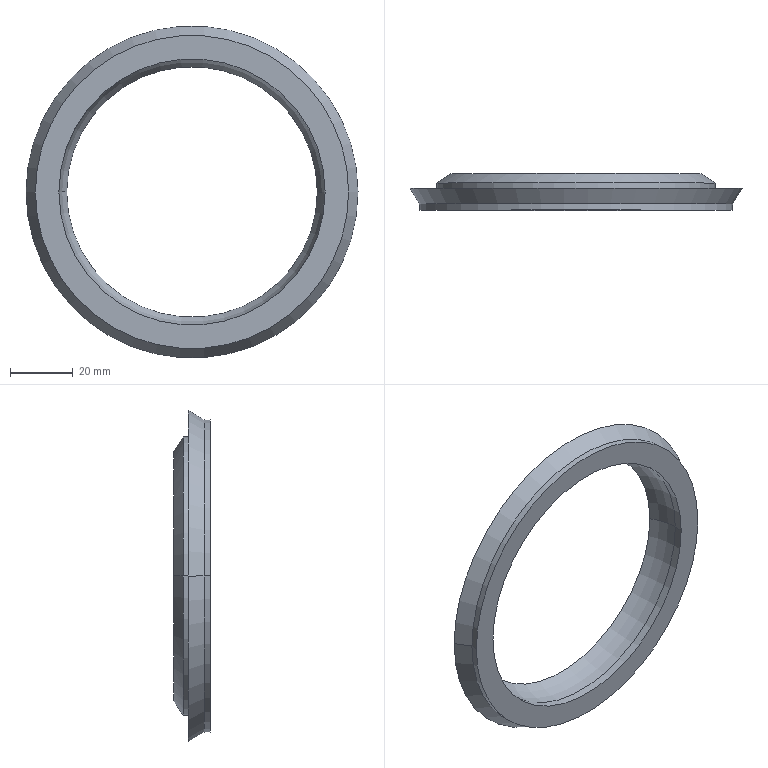Part | SolidWorks | features Revolution 1 | 1 solid | 18 faces | box 106 x 11.67 x 106 mm | volume 13391 mm3 | cylinder 6 | cone 6 | torus 4 | plane 2 | commonest cylinder face diameters 85 x2 89 x2 99.991 x2
STEP:
#1=CARTESIAN_POINT('',(-42.5,-3.5,0.));
#2=VERTEX_POINT('',#1);
#3=CARTESIAN_POINT('',(42.5,-3.5,0.));
#4=VERTEX_POINT('',#3);
#5=CARTESIAN_POINT('',(0.,-3.5,0.));
#6=DIRECTION('',(0.,-1.,0.));
#7=DIRECTION('',(1.,0.,0.));
#8=AXIS2_PLACEMENT_3D('',#5,#6,#7);
#9=CIRCLE('',#8,42.5);
#10=EDGE_CURVE('',#2,#4,#9,.T.);
#11=ORIENTED_EDGE('',*,*,#10,.F.);
#12=CARTESIAN_POINT('',(-42.5,-6.17,0.));
#13=VERTEX_POINT('',#12);
#14=CARTESIAN_POINT('',(-42.5,-5.5,0.));
#15=DIRECTION('',(0.,-1.,0.));
#16=VECTOR('',#15,1000.);
#17=LINE('',#14,#16);
#18=EDGE_CURVE('',#2,#13,#17,.T.);
#19=ORIENTED_EDGE('',*,*,#18,.T.);
#20=CARTESIAN_POINT('',(42.5,-6.17,0.));
#21=VERTEX_POINT('',#20);
#22=CARTESIAN_POINT('',(0.,-6.17,0.));
#23=DIRECTION('',(0.,-1.,0.));
#24=DIRECTION('',(1.,0.,0.));
#25=AXIS2_PLACEMENT_3D('',#22,#23,#24);
#26=CIRCLE('',#25,42.5);
#27=EDGE_CURVE('',#13,#21,#26,.T.);
#28=ORIENTED_EDGE('',*,*,#27,.T.);
#29=CARTESIAN_POINT('',(42.5,-5.5,0.));
#30=DIRECTION('',(0.,-1.,0.));
#31=VECTOR('',#30,1000.);
#32=LINE('',#29,#31);
#33=EDGE_CURVE('',#4,#21,#32,.T.);
#34=ORIENTED_EDGE('',*,*,#33,.F.);
#35=EDGE_LOOP('',(#11,#19,#28,#34));
#36=FACE_OUTER_BOUND('',#35,.T.);
#37=CARTESIAN_POINT('',(0.,-5.5,0.));
#38=DIRECTION('',(0.,-1.,0.));
#39=DIRECTION('',(1.,0.,0.));
#40=AXIS2_PLACEMENT_3D('',#37,#38,#39);
#41=CYLINDRICAL_SURFACE('',#40,42.5);
#42=ADVANCED_FACE('',(#36),#41,.F.);
#43=CARTESIAN_POINT('',(-40.,5.5,0.));
#44=VERTEX_POINT('',#43);
#45=CARTESIAN_POINT('',(40.,5.5,0.));
#46=VERTEX_POINT('',#45);
#47=CARTESIAN_POINT('',(0.,5.5,0.));
#48=DIRECTION('',(0.,-1.,0.));
#49=DIRECTION('',(1.,0.,0.));
#50=AXIS2_PLACEMENT_3D('',#47,#48,#49);
#51=CIRCLE('',#50,40.);
#52=EDGE_CURVE('',#44,#46,#51,.T.);
#53=ORIENTED_EDGE('',*,*,#52,.F.);
#54=CARTESIAN_POINT('',(-27.516,-2.815,0.));
#55=DIRECTION('',(0.,0.,1.));
#56=DIRECTION('',(1.,0.,0.));
#57=AXIS2_PLACEMENT_3D('',#54,#55,#56);
#58=CIRCLE('',#57,15.);
#59=EDGE_CURVE('',#44,#2,#58,.T.);
#60=ORIENTED_EDGE('',*,*,#59,.T.);
#61=ORIENTED_EDGE('',*,*,#10,.T.);
#62=CARTESIAN_POINT('',(27.516,-2.815,0.));
#63=DIRECTION('',(0.,0.,-1.));
#64=DIRECTION('',(-1.,0.,0.));
#65=AXIS2_PLACEMENT_3D('',#62,#63,#64);
#66=CIRCLE('',#65,15.);
#67=EDGE_CURVE('',#46,#4,#66,.T.);
#68=ORIENTED_EDGE('',*,*,#67,.F.);
#69=EDGE_LOOP('',(#53,#60,#61,#68));
#70=FACE_OUTER_BOUND('',#69,.T.);
#71=CARTESIAN_POINT('',(0.,-2.815,0.));
#72=DIRECTION('',(0.,-1.,0.));
#73=DIRECTION('',(1.,0.,0.));
#74=AXIS2_PLACEMENT_3D('',#71,#72,#73);
#75=TOROIDAL_SURFACE('',#74,27.516,15.);
#76=ADVANCED_FACE('',(#70),#75,.F.);
#77=CARTESIAN_POINT('',(0.,5.5,0.));
#78=DIRECTION('',(0.,-1.,0.));
#79=DIRECTION('',(1.,0.,0.));
#80=AXIS2_PLACEMENT_3D('',#77,#78,#79);
#81=CIRCLE('',#80,40.);
#82=EDGE_CURVE('',#46,#44,#81,.T.);
#83=ORIENTED_EDGE('',*,*,#82,.T.);
#84=CARTESIAN_POINT('',(-44.5,2.5,0.));
#85=VERTEX_POINT('',#84);
#86=CARTESIAN_POINT('',(-44.5,2.5,0.));
#87=DIRECTION('',(-0.8321,-0.5547,0.));
#88=VECTOR('',#87,1000.);
#89=LINE('',#86,#88);
#90=EDGE_CURVE('',#44,#85,#89,.T.);
#91=ORIENTED_EDGE('',*,*,#90,.T.);
#92=CARTESIAN_POINT('',(44.5,2.5,0.));
#93=VERTEX_POINT('',#92);
#94=CARTESIAN_POINT('',(0.,2.5,0.));
#95=DIRECTION('',(0.,-1.,0.));
#96=DIRECTION('',(1.,0.,0.));
#97=AXIS2_PLACEMENT_3D('',#94,#95,#96);
#98=CIRCLE('',#97,44.5);
#99=EDGE_CURVE('',#93,#85,#98,.T.);
#100=ORIENTED_EDGE('',*,*,#99,.F.);
#101=CARTESIAN_POINT('',(44.5,2.5,0.));
#102=DIRECTION('',(0.8321,-0.5547,0.));
#103=VECTOR('',#102,1000.);
#104=LINE('',#101,#103);
#105=EDGE_CURVE('',#46,#93,#104,.T.);
#106=ORIENTED_EDGE('',*,*,#105,.F.);
#107=EDGE_LOOP('',(#83,#91,#100,#106));
#108=FACE_OUTER_BOUND('',#107,.T.);
#109=CARTESIAN_POINT('',(0.,2.5,0.));
#110=DIRECTION('',(0.,-1.,0.));
#111=DIRECTION('',(1.,0.,0.));
#112=AXIS2_PLACEMENT_3D('',#109,#110,#111);
#113=CONICAL_SURFACE('',#112,44.5,0.9828);
#114=ADVANCED_FACE('',(#108),#113,.T.);
#115=ORIENTED_EDGE('',*,*,#99,.T.);
#116=CARTESIAN_POINT('',(-44.5,-2.5,0.));
#117=VERTEX_POINT('',#116);
#118=CARTESIAN_POINT('',(-44.5,-5.5,0.));
#119=DIRECTION('',(0.,-1.,0.));
#120=VECTOR('',#119,1000.);
#121=LINE('',#118,#120);
#122=EDGE_CURVE('',#85,#117,#121,.T.);
#123=ORIENTED_EDGE('',*,*,#122,.T.);
#124=CARTESIAN_POINT('',(44.5,-2.5,0.));
#125=VERTEX_POINT('',#124);
#126=CARTESIAN_POINT('',(0.,-2.5,0.));
#127=DIRECTION('',(0.,-1.,0.));
#128=DIRECTION('',(1.,0.,0.));
#129=AXIS2_PLACEMENT_3D('',#126,#127,#128);
#130=CIRCLE('',#129,44.5);
#131=EDGE_CURVE('',#125,#117,#130,.T.);
#132=ORIENTED_EDGE('',*,*,#131,.F.);
#133=CARTESIAN_POINT('',(44.5,-5.5,0.));
#134=DIRECTION('',(0.,-1.,0.));
#135=VECTOR('',#134,1000.);
#136=LINE('',#133,#135);
#137=EDGE_CURVE('',#93,#125,#136,.T.);
#138=ORIENTED_EDGE('',*,*,#137,.F.);
#139=EDGE_LOOP('',(#115,#123,#132,#138));
#140=FACE_OUTER_BOUND('',#139,.T.);
#141=CARTESIAN_POINT('',(0.,-5.5,0.));
#142=DIRECTION('',(0.,-1.,0.));
#143=DIRECTION('',(1.,0.,0.));
#144=AXIS2_PLACEMENT_3D('',#141,#142,#143);
#145=CYLINDRICAL_SURFACE('',#144,44.5);
#146=ADVANCED_FACE('',(#140),#145,.T.);
#147=CARTESIAN_POINT('',(-45.5,-3.5,0.));
#148=VERTEX_POINT('',#147);
#149=CARTESIAN_POINT('',(45.5,-3.5,0.));
#150=VERTEX_POINT('',#149);
#151=CARTESIAN_POINT('',(0.,-3.5,0.));
#152=DIRECTION('',(0.,-1.,0.));
#153=DIRECTION('',(1.,0.,0.));
#154=AXIS2_PLACEMENT_3D('',#151,#152,#153);
#155=CIRCLE('',#154,45.5);
#156=EDGE_CURVE('',#148,#150,#155,.T.);
#157=ORIENTED_EDGE('',*,*,#156,.F.);
#158=CARTESIAN_POINT('',(-45.5,-2.5,0.));
#159=DIRECTION('',(0.,0.,1.));
#160=DIRECTION('',(1.,0.,0.));
#161=AXIS2_PLACEMENT_3D('',#158,#159,#160);
#162=CIRCLE('',#161,1.);
#163=EDGE_CURVE('',#148,#117,#162,.T.);
#164=ORIENTED_EDGE('',*,*,#163,.T.);
#165=CARTESIAN_POINT('',(0.,-2.5,0.));
#166=DIRECTION('',(0.,-1.,0.));
#167=DIRECTION('',(1.,0.,0.));
#168=AXIS2_PLACEMENT_3D('',#165,#166,#167);
#169=CIRCLE('',#168,44.5);
#170=EDGE_CURVE('',#117,#125,#169,.T.);
#171=ORIENTED_EDGE('',*,*,#170,.T.);
#172=CARTESIAN_POINT('',(45.5,-2.5,0.));
#173=DIRECTION('',(0.,0.,-1.));
#174=DIRECTION('',(-1.,0.,0.));
#175=AXIS2_PLACEMENT_3D('',#172,#173,#174);
#176=CIRCLE('',#175,1.);
#177=EDGE_CURVE('',#150,#125,#176,.T.);
#178=ORIENTED_EDGE('',*,*,#177,.F.);
#179=EDGE_LOOP('',(#157,#164,#171,#178));
#180=FACE_OUTER_BOUND('',#179,.T.);
#181=CARTESIAN_POINT('',(0.,-2.5,0.));
#182=DIRECTION('',(0.,-1.,0.));
#183=DIRECTION('',(1.,0.,0.));
#184=AXIS2_PLACEMENT_3D('',#181,#182,#183);
#185=TOROIDAL_SURFACE('',#184,45.5,1.);
#186=ADVANCED_FACE('',(#180),#185,.F.);
#187=CARTESIAN_POINT('',(-46.5,-3.5,0.));
#188=VERTEX_POINT('',#187);
#189=CARTESIAN_POINT('',(46.5,-3.5,0.));
#190=VERTEX_POINT('',#189);
#191=CARTESIAN_POINT('',(0.,-3.5,0.));
#192=DIRECTION('',(0.,-1.,0.));
#193=DIRECTION('',(1.,0.,0.));
#194=AXIS2_PLACEMENT_3D('',#191,#192,#193);
#195=CIRCLE('',#194,46.5);
#196=EDGE_CURVE('',#188,#190,#195,.T.);
#197=ORIENTED_EDGE('',*,*,#196,.T.);
#198=CARTESIAN_POINT('',(53.,0.8301,0.));
#199=VERTEX_POINT('',#198);
#200=CARTESIAN_POINT('',(53.,0.8301,0.));
#201=DIRECTION('',(0.8322,0.5544,0.));
#202=VECTOR('',#201,1000.);
#203=LINE('',#200,#202);
#204=EDGE_CURVE('',#190,#199,#203,.T.);
#205=ORIENTED_EDGE('',*,*,#204,.T.);
#206=CARTESIAN_POINT('',(-53.,0.8301,0.));
#207=VERTEX_POINT('',#206);
#208=CARTESIAN_POINT('',(0.,0.8301,0.));
#209=DIRECTION('',(0.,-1.,0.));
#210=DIRECTION('',(1.,0.,0.));
#211=AXIS2_PLACEMENT_3D('',#208,#209,#210);
#212=CIRCLE('',#211,53.);
#213=EDGE_CURVE('',#207,#199,#212,.T.);
#214=ORIENTED_EDGE('',*,*,#213,.F.);
#215=CARTESIAN_POINT('',(-53.,0.8301,0.));
#216=DIRECTION('',(-0.8322,0.5544,0.));
#217=VECTOR('',#216,1000.);
#218=LINE('',#215,#217);
#219=EDGE_CURVE('',#188,#207,#218,.T.);
#220=ORIENTED_EDGE('',*,*,#219,.F.);
#221=EDGE_LOOP('',(#197,#205,#214,#220));
#222=FACE_OUTER_BOUND('',#221,.T.);
#223=CARTESIAN_POINT('',(0.,0.8301,0.));
#224=DIRECTION('',(0.,1.,0.));
#225=DIRECTION('',(-1.,0.,0.));
#226=AXIS2_PLACEMENT_3D('',#223,#224,#225);
#227=CONICAL_SURFACE('',#226,53.,0.9831);
#228=ADVANCED_FACE('',(#222),#227,.F.);
#229=CARTESIAN_POINT('',(49.996,-4.17,0.));
#230=VERTEX_POINT('',#229);
#231=CARTESIAN_POINT('',(-49.996,-4.17,0.));
#232=VERTEX_POINT('',#231);
#233=CARTESIAN_POINT('',(0.,-4.17,0.));
#234=DIRECTION('',(0.,-1.,0.));
#235=DIRECTION('',(1.,0.,0.));
#236=AXIS2_PLACEMENT_3D('',#233,#234,#235);
#237=CIRCLE('',#236,49.996);
#238=EDGE_CURVE('',#230,#232,#237,.T.);
#239=ORIENTED_EDGE('',*,*,#238,.F.);
#240=CARTESIAN_POINT('',(49.996,-4.17,0.));
#241=DIRECTION('',(0.5151,0.8572,0.));
#242=VECTOR('',#241,1000.);
#243=LINE('',#240,#242);
#244=EDGE_CURVE('',#230,#199,#243,.T.);
#245=ORIENTED_EDGE('',*,*,#244,.T.);
#246=CARTESIAN_POINT('',(0.,0.8301,0.));
#247=DIRECTION('',(0.,-1.,0.));
#248=DIRECTION('',(1.,0.,0.));
#249=AXIS2_PLACEMENT_3D('',#246,#247,#248);
#250=CIRCLE('',#249,53.);
#251=EDGE_CURVE('',#199,#207,#250,.T.);
#252=ORIENTED_EDGE('',*,*,#251,.T.);
#253=CARTESIAN_POINT('',(-49.996,-4.17,0.));
#254=DIRECTION('',(-0.5151,0.8572,0.));
#255=VECTOR('',#254,1000.);
#256=LINE('',#253,#255);
#257=EDGE_CURVE('',#232,#207,#256,.T.);
#258=ORIENTED_EDGE('',*,*,#257,.F.);
#259=EDGE_LOOP('',(#239,#245,#252,#258));
#260=FACE_OUTER_BOUND('',#259,.T.);
#261=CARTESIAN_POINT('',(0.,-4.17,0.));
#262=DIRECTION('',(0.,1.,0.));
#263=DIRECTION('',(-1.,0.,0.));
#264=AXIS2_PLACEMENT_3D('',#261,#262,#263);
#265=CONICAL_SURFACE('',#264,49.996,0.5411);
#266=ADVANCED_FACE('',(#260),#265,.T.);
#267=ORIENTED_EDGE('',*,*,#238,.T.);
#268=CARTESIAN_POINT('',(-49.996,-6.17,0.));
#269=VERTEX_POINT('',#268);
#270=CARTESIAN_POINT('',(-49.996,-5.5,0.));
#271=DIRECTION('',(0.,-1.,0.));
#272=VECTOR('',#271,1000.);
#273=LINE('',#270,#272);
#274=EDGE_CURVE('',#232,#269,#273,.T.);
#275=ORIENTED_EDGE('',*,*,#274,.T.);
#276=CARTESIAN_POINT('',(49.996,-6.17,0.));
#277=VERTEX_POINT('',#276);
#278=CARTESIAN_POINT('',(0.,-6.17,0.));
#279=DIRECTION('',(0.,-1.,0.));
#280=DIRECTION('',(1.,0.,0.));
#281=AXIS2_PLACEMENT_3D('',#278,#279,#280);
#282=CIRCLE('',#281,49.996);
#283=EDGE_CURVE('',#277,#269,#282,.T.);
#284=ORIENTED_EDGE('',*,*,#283,.F.);
#285=CARTESIAN_POINT('',(49.996,-5.5,0.));
#286=DIRECTION('',(0.,-1.,0.));
#287=VECTOR('',#286,1000.);
#288=LINE('',#285,#287);
#289=EDGE_CURVE('',#230,#277,#288,.T.);
#290=ORIENTED_EDGE('',*,*,#289,.F.);
#291=EDGE_LOOP('',(#267,#275,#284,#290));
#292=FACE_OUTER_BOUND('',#291,.T.);
#293=CARTESIAN_POINT('',(0.,-5.5,0.));
#294=DIRECTION('',(0.,-1.,0.));
#295=DIRECTION('',(1.,0.,0.));
#296=AXIS2_PLACEMENT_3D('',#293,#294,#295);
#297=CYLINDRICAL_SURFACE('',#296,49.996);
#298=ADVANCED_FACE('',(#292),#297,.T.);
#299=ORIENTED_EDGE('',*,*,#274,.F.);
#300=CARTESIAN_POINT('',(0.,-4.17,0.));
#301=DIRECTION('',(0.,-1.,0.));
#302=DIRECTION('',(1.,0.,0.));
#303=AXIS2_PLACEMENT_3D('',#300,#301,#302);
#304=CIRCLE('',#303,49.996);
#305=EDGE_CURVE('',#232,#230,#304,.T.);
#306=ORIENTED_EDGE('',*,*,#305,.T.);
#307=ORIENTED_EDGE('',*,*,#289,.T.);
#308=CARTESIAN_POINT('',(0.,-6.17,0.));
#309=DIRECTION('',(0.,-1.,0.));
#310=DIRECTION('',(1.,0.,0.));
#311=AXIS2_PLACEMENT_3D('',#308,#309,#310);
#312=CIRCLE('',#311,49.996);
#313=EDGE_CURVE('',#269,#277,#312,.T.);
#314=ORIENTED_EDGE('',*,*,#313,.F.);
#315=EDGE_LOOP('',(#299,#306,#307,#314));
#316=FACE_OUTER_BOUND('',#315,.T.);
#317=CARTESIAN_POINT('',(0.,-5.5,0.));
#318=DIRECTION('',(0.,-1.,0.));
#319=DIRECTION('',(1.,0.,0.));
#320=AXIS2_PLACEMENT_3D('',#317,#318,#319);
#321=CYLINDRICAL_SURFACE('',#320,49.996);
#322=ADVANCED_FACE('',(#316),#321,.T.);
#323=ORIENTED_EDGE('',*,*,#244,.F.);
#324=ORIENTED_EDGE('',*,*,#305,.F.);
#325=ORIENTED_EDGE('',*,*,#257,.T.);
#326=ORIENTED_EDGE('',*,*,#213,.T.);
#327=EDGE_LOOP('',(#323,#324,#325,#326));
#328=FACE_OUTER_BOUND('',#327,.T.);
#329=CARTESIAN_POINT('',(0.,-4.17,0.));
#330=DIRECTION('',(0.,1.,0.));
#331=DIRECTION('',(-1.,0.,0.));
#332=AXIS2_PLACEMENT_3D('',#329,#330,#331);
#333=CONICAL_SURFACE('',#332,49.996,0.5411);
#334=ADVANCED_FACE('',(#328),#333,.T.);
#335=ORIENTED_EDGE('',*,*,#204,.F.);
#336=CARTESIAN_POINT('',(0.,-3.5,0.));
#337=DIRECTION('',(0.,-1.,0.));
#338=DIRECTION('',(1.,0.,0.));
#339=AXIS2_PLACEMENT_3D('',#336,#337,#338);
#340=CIRCLE('',#339,46.5);
#341=EDGE_CURVE('',#190,#188,#340,.T.);
#342=ORIENTED_EDGE('',*,*,#341,.T.);
#343=ORIENTED_EDGE('',*,*,#219,.T.);
#344=ORIENTED_EDGE('',*,*,#251,.F.);
#345=EDGE_LOOP('',(#335,#342,#343,#344));
#346=FACE_OUTER_BOUND('',#345,.T.);
#347=CARTESIAN_POINT('',(0.,0.8301,0.));
#348=DIRECTION('',(0.,1.,0.));
#349=DIRECTION('',(-1.,0.,0.));
#350=AXIS2_PLACEMENT_3D('',#347,#348,#349);
#351=CONICAL_SURFACE('',#350,53.,0.9831);
#352=ADVANCED_FACE('',(#346),#351,.F.);
#353=CARTESIAN_POINT('',(0.,-3.5,0.));
#354=DIRECTION('',(0.,-1.,0.));
#355=DIRECTION('',(1.,0.,0.));
#356=AXIS2_PLACEMENT_3D('',#353,#354,#355);
#357=CIRCLE('',#356,45.5);
#358=EDGE_CURVE('',#150,#148,#357,.T.);
#359=ORIENTED_EDGE('',*,*,#358,.T.);
#360=ORIENTED_EDGE('',*,*,#156,.T.);
#361=EDGE_LOOP('',(#359,#360));
#362=FACE_BOUND('',#361,.T.);
#363=ORIENTED_EDGE('',*,*,#196,.F.);
#364=ORIENTED_EDGE('',*,*,#341,.F.);
#365=EDGE_LOOP('',(#363,#364));
#366=FACE_OUTER_BOUND('',#365,.T.);
#367=CARTESIAN_POINT('',(46.5,-3.5,0.));
#368=DIRECTION('',(0.,1.,0.));
#369=DIRECTION('',(-1.,0.,0.));
#370=AXIS2_PLACEMENT_3D('',#367,#368,#369);
#371=PLANE('',#370);
#372=ADVANCED_FACE('',(#362,#366),#371,.T.);
#373=ORIENTED_EDGE('',*,*,#163,.F.);
#374=ORIENTED_EDGE('',*,*,#358,.F.);
#375=ORIENTED_EDGE('',*,*,#177,.T.);
#376=ORIENTED_EDGE('',*,*,#131,.T.);
#377=EDGE_LOOP('',(#373,#374,#375,#376));
#378=FACE_OUTER_BOUND('',#377,.T.);
#379=CARTESIAN_POINT('',(0.,-2.5,0.));
#380=DIRECTION('',(0.,-1.,0.));
#381=DIRECTION('',(1.,0.,0.));
#382=AXIS2_PLACEMENT_3D('',#379,#380,#381);
#383=TOROIDAL_SURFACE('',#382,45.5,1.);
#384=ADVANCED_FACE('',(#378),#383,.F.);
#385=ORIENTED_EDGE('',*,*,#122,.F.);
#386=CARTESIAN_POINT('',(0.,2.5,0.));
#387=DIRECTION('',(0.,-1.,0.));
#388=DIRECTION('',(1.,0.,0.));
#389=AXIS2_PLACEMENT_3D('',#386,#387,#388);
#390=CIRCLE('',#389,44.5);
#391=EDGE_CURVE('',#85,#93,#390,.T.);
#392=ORIENTED_EDGE('',*,*,#391,.T.);
#393=ORIENTED_EDGE('',*,*,#137,.T.);
#394=ORIENTED_EDGE('',*,*,#170,.F.);
#395=EDGE_LOOP('',(#385,#392,#393,#394));
#396=FACE_OUTER_BOUND('',#395,.T.);
#397=CARTESIAN_POINT('',(0.,-5.5,0.));
#398=DIRECTION('',(0.,-1.,0.));
#399=DIRECTION('',(1.,0.,0.));
#400=AXIS2_PLACEMENT_3D('',#397,#398,#399);
#401=CYLINDRICAL_SURFACE('',#400,44.5);
#402=ADVANCED_FACE('',(#396),#401,.T.);
#403=ORIENTED_EDGE('',*,*,#90,.F.);
#404=ORIENTED_EDGE('',*,*,#52,.T.);
#405=ORIENTED_EDGE('',*,*,#105,.T.);
#406=ORIENTED_EDGE('',*,*,#391,.F.);
#407=EDGE_LOOP('',(#403,#404,#405,#406));
#408=FACE_OUTER_BOUND('',#407,.T.);
#409=CARTESIAN_POINT('',(0.,2.5,0.));
#410=DIRECTION('',(0.,-1.,0.));
#411=DIRECTION('',(1.,0.,0.));
#412=AXIS2_PLACEMENT_3D('',#409,#410,#411);
#413=CONICAL_SURFACE('',#412,44.5,0.9828);
#414=ADVANCED_FACE('',(#408),#413,.T.);
#415=ORIENTED_EDGE('',*,*,#59,.F.);
#416=ORIENTED_EDGE('',*,*,#82,.F.);
#417=ORIENTED_EDGE('',*,*,#67,.T.);
#418=CARTESIAN_POINT('',(0.,-3.5,0.));
#419=DIRECTION('',(0.,-1.,0.));
#420=DIRECTION('',(1.,0.,0.));
#421=AXIS2_PLACEMENT_3D('',#418,#419,#420);
#422=CIRCLE('',#421,42.5);
#423=EDGE_CURVE('',#4,#2,#422,.T.);
#424=ORIENTED_EDGE('',*,*,#423,.T.);
#425=EDGE_LOOP('',(#415,#416,#417,#424));
#426=FACE_OUTER_BOUND('',#425,.T.);
#427=CARTESIAN_POINT('',(0.,-2.815,0.));
#428=DIRECTION('',(0.,-1.,0.));
#429=DIRECTION('',(1.,0.,0.));
#430=AXIS2_PLACEMENT_3D('',#427,#428,#429);
#431=TOROIDAL_SURFACE('',#430,27.516,15.);
#432=ADVANCED_FACE('',(#426),#431,.F.);
#433=ORIENTED_EDGE('',*,*,#18,.F.);
#434=ORIENTED_EDGE('',*,*,#423,.F.);
#435=ORIENTED_EDGE('',*,*,#33,.T.);
#436=CARTESIAN_POINT('',(0.,-6.17,0.));
#437=DIRECTION('',(0.,-1.,0.));
#438=DIRECTION('',(1.,0.,0.));
#439=AXIS2_PLACEMENT_3D('',#436,#437,#438);
#440=CIRCLE('',#439,42.5);
#441=EDGE_CURVE('',#21,#13,#440,.T.);
#442=ORIENTED_EDGE('',*,*,#441,.T.);
#443=EDGE_LOOP('',(#433,#434,#435,#442));
#444=FACE_OUTER_BOUND('',#443,.T.);
#445=CARTESIAN_POINT('',(0.,-5.5,0.));
#446=DIRECTION('',(0.,-1.,0.));
#447=DIRECTION('',(1.,0.,0.));
#448=AXIS2_PLACEMENT_3D('',#445,#446,#447);
#449=CYLINDRICAL_SURFACE('',#448,42.5);
#450=ADVANCED_FACE('',(#444),#449,.F.);
#451=ORIENTED_EDGE('',*,*,#283,.T.);
#452=ORIENTED_EDGE('',*,*,#313,.T.);
#453=EDGE_LOOP('',(#451,#452));
#454=FACE_OUTER_BOUND('',#453,.T.);
#455=ORIENTED_EDGE('',*,*,#441,.F.);
#456=ORIENTED_EDGE('',*,*,#27,.F.);
#457=EDGE_LOOP('',(#455,#456));
#458=FACE_BOUND('',#457,.T.);
#459=CARTESIAN_POINT('',(42.5,-6.17,0.));
#460=DIRECTION('',(0.,-1.,0.));
#461=DIRECTION('',(1.,0.,0.));
#462=AXIS2_PLACEMENT_3D('',#459,#460,#461);
#463=PLANE('',#462);
#464=ADVANCED_FACE('',(#454,#458),#463,.T.);
#465=CLOSED_SHELL('',(#42,#76,#114,#146,#186,#228,#266,#298,#322,#334,#352,#372,#384,#402,#414,#432,#450,#464));
#466=MANIFOLD_SOLID_BREP('',#465);
#467=CARTESIAN_POINT('',(0.,0.,0.));
#468=DIRECTION('',(0.,0.,1.));
#469=DIRECTION('',(1.,0.,0.));
#470=AXIS2_PLACEMENT_3D('',#467,#468,#469);
#471=(LENGTH_UNIT()NAMED_UNIT(*)SI_UNIT(.MILLI.,.METRE.));
#472=UNCERTAINTY_MEASURE_WITH_UNIT(LENGTH_MEASURE(0.00001),#471,'','');
#473=(NAMED_UNIT(*)PLANE_ANGLE_UNIT()SI_UNIT($,.RADIAN.));
#474=(NAMED_UNIT(*)SI_UNIT($,.STERADIAN.)SOLID_ANGLE_UNIT());
#475=(GEOMETRIC_REPRESENTATION_CONTEXT(3)GLOBAL_UNCERTAINTY_ASSIGNED_CONTEXT((#472))GLOBAL_UNIT_ASSIGNED_CONTEXT((#471,#473,#474))REPRESENTATION_CONTEXT('',''));
#476=ADVANCED_BREP_SHAPE_REPRESENTATION('',(#466,#470),#475);